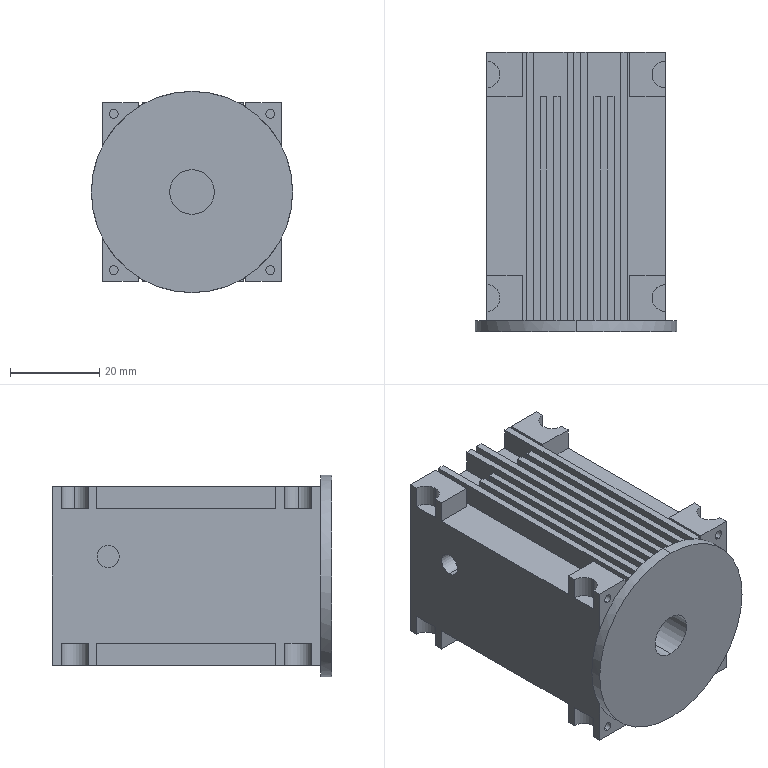Part | SolidWorks | features ICE 8, MirrorPattern 3, Extrusion 1 | 1 solid | 150 faces | box 45 x 62.5 x 45 mm | volume 83715 mm3 | plane 124 | cylinder 26 | commonest cylinder face diameters 6 x12 2 x8 5 x2 10 x2 45 x2